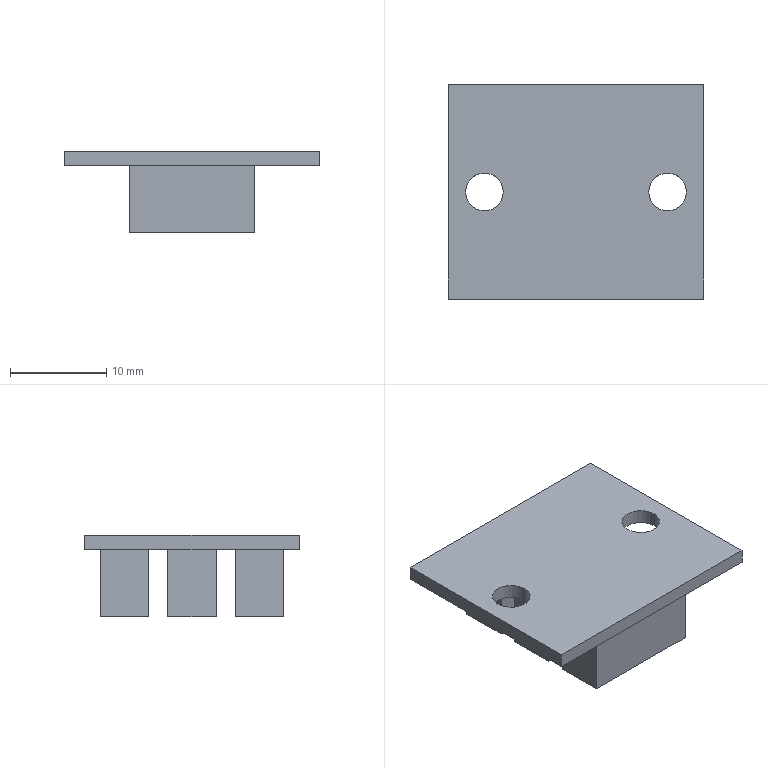Part | STEP file | LJ-sensor2 circuit board V1.0 | 1 solid | 40 faces | box 26.5 x 22.2 x 8.5 mm | volume 1722 mm3 | plane 36 | cylinder 4 | commonest cylinder face diameters 3.9 x4